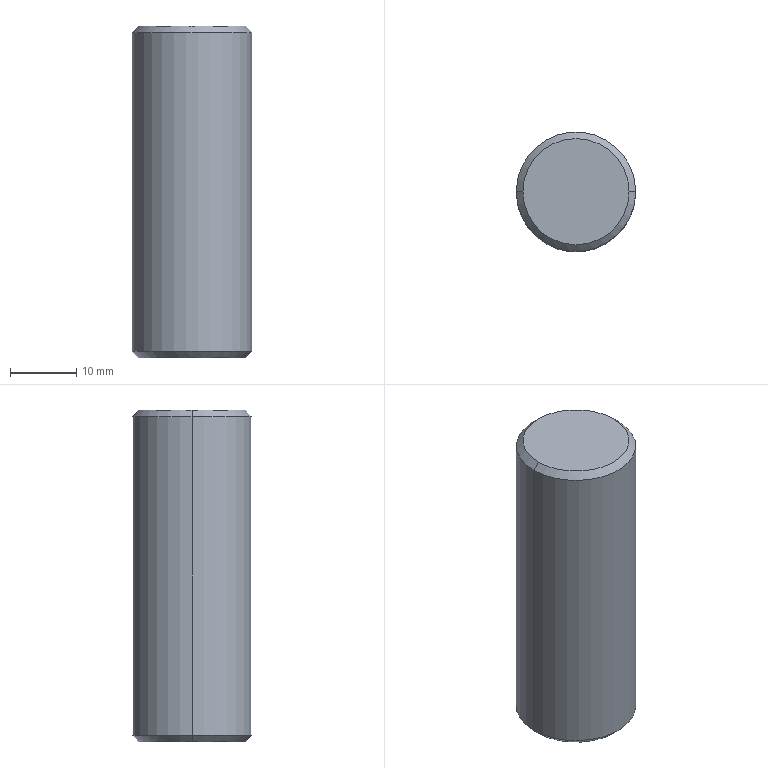Part | SolidWorks | features Chamfer 1, Extrusion 1 | 1 solid | 8 faces | box 18 x 18 x 50 mm | volume 12669 mm3 | cone 4 | cylinder 2 | plane 2 | commonest cylinder face diameters 18 x2
STEP:
#1=CARTESIAN_POINT('',(8.,0.,50.));
#2=VERTEX_POINT('',#1);
#3=CARTESIAN_POINT('',(-8.,0.,50.));
#4=VERTEX_POINT('',#3);
#5=CARTESIAN_POINT('',(0.,0.,50.));
#6=DIRECTION('',(0.,0.,1.));
#7=DIRECTION('',(1.,0.,0.));
#8=AXIS2_PLACEMENT_3D('',#5,#6,#7);
#9=CIRCLE('',#8,8.);
#10=EDGE_CURVE('',#2,#4,#9,.T.);
#11=ORIENTED_EDGE('',*,*,#10,.F.);
#12=CARTESIAN_POINT('',(9.,0.,49.));
#13=VERTEX_POINT('',#12);
#14=CARTESIAN_POINT('',(8.,0.,50.));
#15=DIRECTION('',(0.7071,0.,-0.7071));
#16=VECTOR('',#15,1000.);
#17=LINE('',#14,#16);
#18=EDGE_CURVE('',#2,#13,#17,.T.);
#19=ORIENTED_EDGE('',*,*,#18,.T.);
#20=CARTESIAN_POINT('',(-9.,0.,49.));
#21=VERTEX_POINT('',#20);
#22=CARTESIAN_POINT('',(0.,0.,49.));
#23=DIRECTION('',(0.,0.,-1.));
#24=DIRECTION('',(1.,0.,0.));
#25=AXIS2_PLACEMENT_3D('',#22,#23,#24);
#26=CIRCLE('',#25,9.);
#27=EDGE_CURVE('',#21,#13,#26,.T.);
#28=ORIENTED_EDGE('',*,*,#27,.F.);
#29=CARTESIAN_POINT('',(-8.,0.,50.));
#30=DIRECTION('',(-0.7071,0.,-0.7071));
#31=VECTOR('',#30,1000.);
#32=LINE('',#29,#31);
#33=EDGE_CURVE('',#4,#21,#32,.T.);
#34=ORIENTED_EDGE('',*,*,#33,.F.);
#35=EDGE_LOOP('',(#11,#19,#28,#34));
#36=FACE_OUTER_BOUND('',#35,.T.);
#37=CARTESIAN_POINT('',(0.,0.,50.));
#38=DIRECTION('',(0.,0.,-1.));
#39=DIRECTION('',(-1.,0.,0.));
#40=AXIS2_PLACEMENT_3D('',#37,#38,#39);
#41=CONICAL_SURFACE('',#40,8.,0.7854);
#42=ADVANCED_FACE('',(#36),#41,.T.);
#43=CARTESIAN_POINT('',(-8.,0.,0.));
#44=VERTEX_POINT('',#43);
#45=CARTESIAN_POINT('',(8.,0.,0.));
#46=VERTEX_POINT('',#45);
#47=CARTESIAN_POINT('',(0.,0.,0.));
#48=DIRECTION('',(0.,0.,-1.));
#49=DIRECTION('',(1.,0.,0.));
#50=AXIS2_PLACEMENT_3D('',#47,#48,#49);
#51=CIRCLE('',#50,8.);
#52=EDGE_CURVE('',#44,#46,#51,.T.);
#53=ORIENTED_EDGE('',*,*,#52,.F.);
#54=CARTESIAN_POINT('',(-9.,0.,1.));
#55=VERTEX_POINT('',#54);
#56=CARTESIAN_POINT('',(-9.,0.,1.));
#57=DIRECTION('',(-0.7071,0.,0.7071));
#58=VECTOR('',#57,1000.);
#59=LINE('',#56,#58);
#60=EDGE_CURVE('',#44,#55,#59,.T.);
#61=ORIENTED_EDGE('',*,*,#60,.T.);
#62=CARTESIAN_POINT('',(9.,0.,1.));
#63=VERTEX_POINT('',#62);
#64=CARTESIAN_POINT('',(0.,0.,1.));
#65=DIRECTION('',(0.,0.,1.));
#66=DIRECTION('',(1.,0.,0.));
#67=AXIS2_PLACEMENT_3D('',#64,#65,#66);
#68=CIRCLE('',#67,9.);
#69=EDGE_CURVE('',#63,#55,#68,.T.);
#70=ORIENTED_EDGE('',*,*,#69,.F.);
#71=CARTESIAN_POINT('',(9.,0.,1.));
#72=DIRECTION('',(0.7071,0.,0.7071));
#73=VECTOR('',#72,1000.);
#74=LINE('',#71,#73);
#75=EDGE_CURVE('',#46,#63,#74,.T.);
#76=ORIENTED_EDGE('',*,*,#75,.F.);
#77=EDGE_LOOP('',(#53,#61,#70,#76));
#78=FACE_OUTER_BOUND('',#77,.T.);
#79=CARTESIAN_POINT('',(0.,0.,1.));
#80=DIRECTION('',(0.,0.,1.));
#81=DIRECTION('',(1.,0.,0.));
#82=AXIS2_PLACEMENT_3D('',#79,#80,#81);
#83=CONICAL_SURFACE('',#82,9.,0.7854);
#84=ADVANCED_FACE('',(#78),#83,.T.);
#85=ORIENTED_EDGE('',*,*,#27,.T.);
#86=CARTESIAN_POINT('',(9.,0.,50.));
#87=DIRECTION('',(0.,0.,-1.));
#88=VECTOR('',#87,1000.);
#89=LINE('',#86,#88);
#90=EDGE_CURVE('',#13,#63,#89,.T.);
#91=ORIENTED_EDGE('',*,*,#90,.T.);
#92=ORIENTED_EDGE('',*,*,#69,.T.);
#93=CARTESIAN_POINT('',(-9.,0.,50.));
#94=DIRECTION('',(0.,0.,-1.));
#95=VECTOR('',#94,1000.);
#96=LINE('',#93,#95);
#97=EDGE_CURVE('',#21,#55,#96,.T.);
#98=ORIENTED_EDGE('',*,*,#97,.F.);
#99=EDGE_LOOP('',(#85,#91,#92,#98));
#100=FACE_OUTER_BOUND('',#99,.T.);
#101=CARTESIAN_POINT('',(0.,0.,50.));
#102=DIRECTION('',(0.,0.,-1.));
#103=DIRECTION('',(-1.,0.,0.));
#104=AXIS2_PLACEMENT_3D('',#101,#102,#103);
#105=CYLINDRICAL_SURFACE('',#104,9.);
#106=ADVANCED_FACE('',(#100),#105,.T.);
#107=ORIENTED_EDGE('',*,*,#90,.F.);
#108=CARTESIAN_POINT('',(0.,0.,49.));
#109=DIRECTION('',(0.,0.,-1.));
#110=DIRECTION('',(1.,0.,0.));
#111=AXIS2_PLACEMENT_3D('',#108,#109,#110);
#112=CIRCLE('',#111,9.);
#113=EDGE_CURVE('',#13,#21,#112,.T.);
#114=ORIENTED_EDGE('',*,*,#113,.T.);
#115=ORIENTED_EDGE('',*,*,#97,.T.);
#116=CARTESIAN_POINT('',(0.,0.,1.));
#117=DIRECTION('',(0.,0.,1.));
#118=DIRECTION('',(1.,0.,0.));
#119=AXIS2_PLACEMENT_3D('',#116,#117,#118);
#120=CIRCLE('',#119,9.);
#121=EDGE_CURVE('',#55,#63,#120,.T.);
#122=ORIENTED_EDGE('',*,*,#121,.T.);
#123=EDGE_LOOP('',(#107,#114,#115,#122));
#124=FACE_OUTER_BOUND('',#123,.T.);
#125=CARTESIAN_POINT('',(0.,0.,50.));
#126=DIRECTION('',(0.,0.,-1.));
#127=DIRECTION('',(-1.,0.,0.));
#128=AXIS2_PLACEMENT_3D('',#125,#126,#127);
#129=CYLINDRICAL_SURFACE('',#128,9.);
#130=ADVANCED_FACE('',(#124),#129,.T.);
#131=CARTESIAN_POINT('',(0.,0.,50.));
#132=DIRECTION('',(0.,0.,1.));
#133=DIRECTION('',(1.,0.,0.));
#134=AXIS2_PLACEMENT_3D('',#131,#132,#133);
#135=CIRCLE('',#134,8.);
#136=EDGE_CURVE('',#4,#2,#135,.T.);
#137=ORIENTED_EDGE('',*,*,#136,.T.);
#138=ORIENTED_EDGE('',*,*,#10,.T.);
#139=EDGE_LOOP('',(#137,#138));
#140=FACE_OUTER_BOUND('',#139,.T.);
#141=CARTESIAN_POINT('',(0.,0.,50.));
#142=DIRECTION('',(0.,0.,1.));
#143=DIRECTION('',(1.,0.,0.));
#144=AXIS2_PLACEMENT_3D('',#141,#142,#143);
#145=PLANE('',#144);
#146=ADVANCED_FACE('',(#140),#145,.T.);
#147=CARTESIAN_POINT('',(0.,0.,0.));
#148=DIRECTION('',(0.,0.,-1.));
#149=DIRECTION('',(1.,0.,0.));
#150=AXIS2_PLACEMENT_3D('',#147,#148,#149);
#151=CIRCLE('',#150,8.);
#152=EDGE_CURVE('',#46,#44,#151,.T.);
#153=ORIENTED_EDGE('',*,*,#152,.T.);
#154=ORIENTED_EDGE('',*,*,#52,.T.);
#155=EDGE_LOOP('',(#153,#154));
#156=FACE_OUTER_BOUND('',#155,.T.);
#157=CARTESIAN_POINT('',(0.,0.,0.));
#158=DIRECTION('',(0.,0.,1.));
#159=DIRECTION('',(1.,0.,0.));
#160=AXIS2_PLACEMENT_3D('',#157,#158,#159);
#161=PLANE('',#160);
#162=ADVANCED_FACE('',(#156),#161,.F.);
#163=ORIENTED_EDGE('',*,*,#60,.F.);
#164=ORIENTED_EDGE('',*,*,#152,.F.);
#165=ORIENTED_EDGE('',*,*,#75,.T.);
#166=ORIENTED_EDGE('',*,*,#121,.F.);
#167=EDGE_LOOP('',(#163,#164,#165,#166));
#168=FACE_OUTER_BOUND('',#167,.T.);
#169=CARTESIAN_POINT('',(0.,0.,1.));
#170=DIRECTION('',(0.,0.,1.));
#171=DIRECTION('',(1.,0.,0.));
#172=AXIS2_PLACEMENT_3D('',#169,#170,#171);
#173=CONICAL_SURFACE('',#172,9.,0.7854);
#174=ADVANCED_FACE('',(#168),#173,.T.);
#175=ORIENTED_EDGE('',*,*,#18,.F.);
#176=ORIENTED_EDGE('',*,*,#136,.F.);
#177=ORIENTED_EDGE('',*,*,#33,.T.);
#178=ORIENTED_EDGE('',*,*,#113,.F.);
#179=EDGE_LOOP('',(#175,#176,#177,#178));
#180=FACE_OUTER_BOUND('',#179,.T.);
#181=CARTESIAN_POINT('',(0.,0.,50.));
#182=DIRECTION('',(0.,0.,-1.));
#183=DIRECTION('',(-1.,0.,0.));
#184=AXIS2_PLACEMENT_3D('',#181,#182,#183);
#185=CONICAL_SURFACE('',#184,8.,0.7854);
#186=ADVANCED_FACE('',(#180),#185,.T.);
#187=CLOSED_SHELL('',(#42,#84,#106,#130,#146,#162,#174,#186));
#188=MANIFOLD_SOLID_BREP('',#187);
#189=CARTESIAN_POINT('',(0.,0.,0.));
#190=DIRECTION('',(0.,0.,1.));
#191=DIRECTION('',(1.,0.,0.));
#192=AXIS2_PLACEMENT_3D('',#189,#190,#191);
#193=(LENGTH_UNIT()NAMED_UNIT(*)SI_UNIT(.MILLI.,.METRE.));
#194=UNCERTAINTY_MEASURE_WITH_UNIT(LENGTH_MEASURE(0.00001),#193,'','');
#195=(NAMED_UNIT(*)PLANE_ANGLE_UNIT()SI_UNIT($,.RADIAN.));
#196=(NAMED_UNIT(*)SI_UNIT($,.STERADIAN.)SOLID_ANGLE_UNIT());
#197=(GEOMETRIC_REPRESENTATION_CONTEXT(3)GLOBAL_UNCERTAINTY_ASSIGNED_CONTEXT((#194))GLOBAL_UNIT_ASSIGNED_CONTEXT((#193,#195,#196))REPRESENTATION_CONTEXT('',''));
#198=ADVANCED_BREP_SHAPE_REPRESENTATION('',(#188,#192),#197);